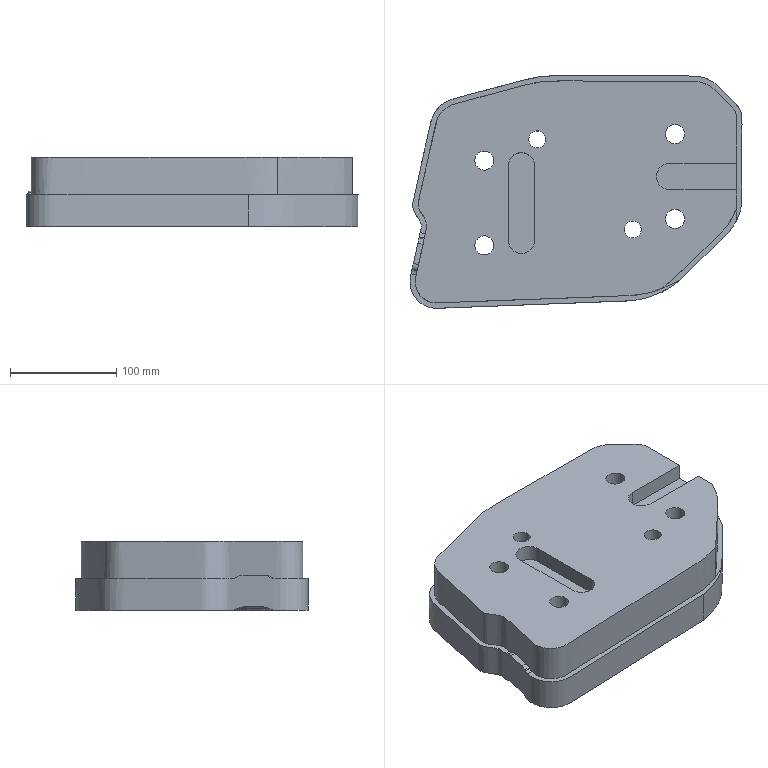Part | NX | features solid 2 | 1 solid | 61 faces | box 313.229 x 219.308 x 65.239 mm | volume 2575726 mm3 | spline 36 | cylinder 13 | plane 12 | commonest cylinder face diameters 18 x4 26 x4 25 x3 16 x2